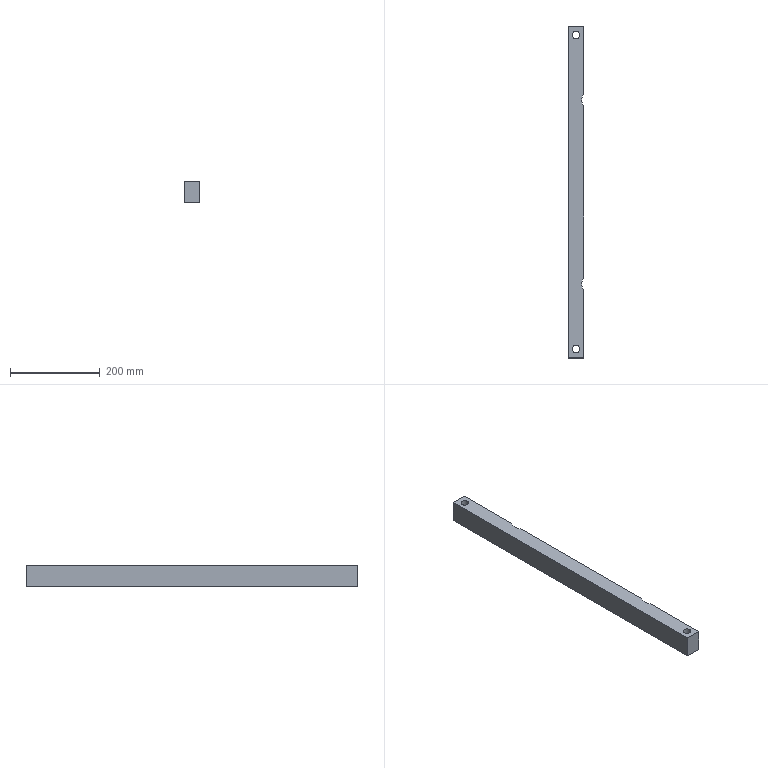Part | NX | features solid 2 | 1 solid | 12 faces | box 35 x 740 x 49 mm | volume 1237665 mm3 | plane 8 | cylinder 4 | commonest cylinder face diameters 17 x2 57 x2
STEP:
#1=CARTESIAN_POINT('',(510.5,-370.,153.));
#2=VERTEX_POINT('',#1);
#3=CARTESIAN_POINT('',(510.5,-370.,202.));
#4=VERTEX_POINT('',#3);
#5=CARTESIAN_POINT('',(510.5,-370.,148.));
#6=DIRECTION('',(0.,0.,1.));
#7=VECTOR('',#6,1000.);
#8=LINE('',#5,#7);
#9=EDGE_CURVE('',#2,#4,#8,.T.);
#10=ORIENTED_EDGE('',*,*,#9,.F.);
#11=CARTESIAN_POINT('',(510.5,-220.37,153.));
#12=VERTEX_POINT('',#11);
#13=CARTESIAN_POINT('',(510.5,0.,153.));
#14=DIRECTION('',(0.,1.,0.));
#15=VECTOR('',#14,1000.);
#16=LINE('',#13,#15);
#17=EDGE_CURVE('',#2,#12,#16,.T.);
#18=ORIENTED_EDGE('',*,*,#17,.T.);
#19=CARTESIAN_POINT('',(510.5,-220.37,202.));
#20=VERTEX_POINT('',#19);
#21=CARTESIAN_POINT('',(510.5,-220.37,308.));
#22=DIRECTION('',(0.,0.,-1.));
#23=VECTOR('',#22,1000.);
#24=LINE('',#21,#23);
#25=EDGE_CURVE('',#12,#20,#24,.F.);
#26=ORIENTED_EDGE('',*,*,#25,.T.);
#27=CARTESIAN_POINT('',(510.5,0.,202.));
#28=DIRECTION('',(0.,-1.,0.));
#29=VECTOR('',#28,1000.);
#30=LINE('',#27,#29);
#31=EDGE_CURVE('',#20,#4,#30,.T.);
#32=ORIENTED_EDGE('',*,*,#31,.T.);
#33=EDGE_LOOP('',(#10,#18,#26,#32));
#34=FACE_BOUND('',#33,.T.);
#35=CARTESIAN_POINT('',(510.5,0.,148.));
#36=DIRECTION('',(1.,0.,0.));
#37=DIRECTION('',(0.,0.,-1.));
#38=AXIS2_PLACEMENT_3D('',#35,#36,#37);
#39=PLANE('',#38);
#40=ADVANCED_FACE('',(#34),#39,.T.);
#41=CARTESIAN_POINT('',(510.5,-189.63,202.));
#42=VERTEX_POINT('',#41);
#43=CARTESIAN_POINT('',(510.5,-189.63,153.));
#44=VERTEX_POINT('',#43);
#45=CARTESIAN_POINT('',(510.5,-189.63,308.));
#46=DIRECTION('',(0.,0.,-1.));
#47=VECTOR('',#46,1000.);
#48=LINE('',#45,#47);
#49=EDGE_CURVE('',#42,#44,#48,.T.);
#50=ORIENTED_EDGE('',*,*,#49,.T.);
#51=CARTESIAN_POINT('',(510.5,189.63,153.));
#52=VERTEX_POINT('',#51);
#53=CARTESIAN_POINT('',(510.5,0.,153.));
#54=DIRECTION('',(0.,1.,0.));
#55=VECTOR('',#54,1000.);
#56=LINE('',#53,#55);
#57=EDGE_CURVE('',#44,#52,#56,.T.);
#58=ORIENTED_EDGE('',*,*,#57,.T.);
#59=CARTESIAN_POINT('',(510.5,189.63,202.));
#60=VERTEX_POINT('',#59);
#61=CARTESIAN_POINT('',(510.5,189.63,308.));
#62=DIRECTION('',(0.,0.,-1.));
#63=VECTOR('',#62,1000.);
#64=LINE('',#61,#63);
#65=EDGE_CURVE('',#52,#60,#64,.F.);
#66=ORIENTED_EDGE('',*,*,#65,.T.);
#67=CARTESIAN_POINT('',(510.5,0.,202.));
#68=DIRECTION('',(0.,-1.,0.));
#69=VECTOR('',#68,1000.);
#70=LINE('',#67,#69);
#71=EDGE_CURVE('',#60,#42,#70,.T.);
#72=ORIENTED_EDGE('',*,*,#71,.T.);
#73=EDGE_LOOP('',(#50,#58,#66,#72));
#74=FACE_BOUND('',#73,.T.);
#75=CARTESIAN_POINT('',(510.5,0.,148.));
#76=DIRECTION('',(1.,0.,0.));
#77=DIRECTION('',(0.,0.,-1.));
#78=AXIS2_PLACEMENT_3D('',#75,#76,#77);
#79=PLANE('',#78);
#80=ADVANCED_FACE('',(#74),#79,.T.);
#81=CARTESIAN_POINT('',(510.5,220.37,202.));
#82=VERTEX_POINT('',#81);
#83=CARTESIAN_POINT('',(510.5,220.37,153.));
#84=VERTEX_POINT('',#83);
#85=CARTESIAN_POINT('',(510.5,220.37,308.));
#86=DIRECTION('',(0.,0.,-1.));
#87=VECTOR('',#86,1000.);
#88=LINE('',#85,#87);
#89=EDGE_CURVE('',#82,#84,#88,.T.);
#90=ORIENTED_EDGE('',*,*,#89,.T.);
#91=CARTESIAN_POINT('',(510.5,370.,153.));
#92=VERTEX_POINT('',#91);
#93=CARTESIAN_POINT('',(510.5,0.,153.));
#94=DIRECTION('',(0.,1.,0.));
#95=VECTOR('',#94,1000.);
#96=LINE('',#93,#95);
#97=EDGE_CURVE('',#84,#92,#96,.T.);
#98=ORIENTED_EDGE('',*,*,#97,.T.);
#99=CARTESIAN_POINT('',(510.5,370.,202.));
#100=VERTEX_POINT('',#99);
#101=CARTESIAN_POINT('',(510.5,370.,148.));
#102=DIRECTION('',(0.,0.,1.));
#103=VECTOR('',#102,1000.);
#104=LINE('',#101,#103);
#105=EDGE_CURVE('',#92,#100,#104,.T.);
#106=ORIENTED_EDGE('',*,*,#105,.T.);
#107=CARTESIAN_POINT('',(510.5,0.,202.));
#108=DIRECTION('',(0.,-1.,0.));
#109=VECTOR('',#108,1000.);
#110=LINE('',#107,#109);
#111=EDGE_CURVE('',#100,#82,#110,.T.);
#112=ORIENTED_EDGE('',*,*,#111,.T.);
#113=EDGE_LOOP('',(#90,#98,#106,#112));
#114=FACE_BOUND('',#113,.T.);
#115=CARTESIAN_POINT('',(510.5,0.,148.));
#116=DIRECTION('',(1.,0.,0.));
#117=DIRECTION('',(0.,0.,-1.));
#118=AXIS2_PLACEMENT_3D('',#115,#116,#117);
#119=PLANE('',#118);
#120=ADVANCED_FACE('',(#114),#119,.T.);
#121=CARTESIAN_POINT('',(484.5,-350.,202.));
#122=VERTEX_POINT('',#121);
#123=CARTESIAN_POINT('',(493.,-350.,202.));
#124=DIRECTION('',(0.,0.,1.));
#125=DIRECTION('',(-1.,0.,0.));
#126=AXIS2_PLACEMENT_3D('',#123,#124,#125);
#127=CIRCLE('',#126,8.5);
#128=EDGE_CURVE('',#122,#122,#127,.F.);
#129=ORIENTED_EDGE('',*,*,#128,.F.);
#130=EDGE_LOOP('',(#129));
#131=FACE_BOUND('',#130,.T.);
#132=CARTESIAN_POINT('',(484.5,-350.,153.));
#133=VERTEX_POINT('',#132);
#134=CARTESIAN_POINT('',(493.,-350.,153.));
#135=DIRECTION('',(0.,0.,-1.));
#136=DIRECTION('',(-1.,0.,0.));
#137=AXIS2_PLACEMENT_3D('',#134,#135,#136);
#138=CIRCLE('',#137,8.5);
#139=EDGE_CURVE('',#133,#133,#138,.F.);
#140=ORIENTED_EDGE('',*,*,#139,.F.);
#141=EDGE_LOOP('',(#140));
#142=FACE_BOUND('',#141,.T.);
#143=CARTESIAN_POINT('',(493.,-350.,202.));
#144=DIRECTION('',(0.,0.,-1.));
#145=DIRECTION('',(-1.,0.,0.));
#146=AXIS2_PLACEMENT_3D('',#143,#144,#145);
#147=CYLINDRICAL_SURFACE('',#146,8.5);
#148=ADVANCED_FACE('',(#131,#142),#147,.F.);
#149=CARTESIAN_POINT('',(475.5,370.,153.));
#150=VERTEX_POINT('',#149);
#151=CARTESIAN_POINT('',(475.5,370.,202.));
#152=VERTEX_POINT('',#151);
#153=CARTESIAN_POINT('',(475.5,370.,148.));
#154=DIRECTION('',(0.,0.,1.));
#155=VECTOR('',#154,1000.);
#156=LINE('',#153,#155);
#157=EDGE_CURVE('',#150,#152,#156,.T.);
#158=ORIENTED_EDGE('',*,*,#157,.F.);
#159=CARTESIAN_POINT('',(475.5,-370.,153.));
#160=VERTEX_POINT('',#159);
#161=CARTESIAN_POINT('',(475.5,0.,153.));
#162=DIRECTION('',(0.,-1.,0.));
#163=VECTOR('',#162,1000.);
#164=LINE('',#161,#163);
#165=EDGE_CURVE('',#150,#160,#164,.T.);
#166=ORIENTED_EDGE('',*,*,#165,.T.);
#167=CARTESIAN_POINT('',(475.5,-370.,202.));
#168=VERTEX_POINT('',#167);
#169=CARTESIAN_POINT('',(475.5,-370.,148.));
#170=DIRECTION('',(0.,0.,1.));
#171=VECTOR('',#170,1000.);
#172=LINE('',#169,#171);
#173=EDGE_CURVE('',#160,#168,#172,.T.);
#174=ORIENTED_EDGE('',*,*,#173,.T.);
#175=CARTESIAN_POINT('',(475.5,0.,202.));
#176=DIRECTION('',(0.,1.,0.));
#177=VECTOR('',#176,1000.);
#178=LINE('',#175,#177);
#179=EDGE_CURVE('',#168,#152,#178,.T.);
#180=ORIENTED_EDGE('',*,*,#179,.T.);
#181=EDGE_LOOP('',(#158,#166,#174,#180));
#182=FACE_BOUND('',#181,.T.);
#183=CARTESIAN_POINT('',(475.5,0.,148.));
#184=DIRECTION('',(-1.,0.,0.));
#185=DIRECTION('',(0.,0.,1.));
#186=AXIS2_PLACEMENT_3D('',#183,#184,#185);
#187=PLANE('',#186);
#188=ADVANCED_FACE('',(#182),#187,.T.);
#189=ORIENTED_EDGE('',*,*,#105,.F.);
#190=CARTESIAN_POINT('',(493.,370.,153.));
#191=DIRECTION('',(-1.,0.,0.));
#192=VECTOR('',#191,1000.);
#193=LINE('',#190,#192);
#194=EDGE_CURVE('',#92,#150,#193,.T.);
#195=ORIENTED_EDGE('',*,*,#194,.T.);
#196=ORIENTED_EDGE('',*,*,#157,.T.);
#197=CARTESIAN_POINT('',(493.,370.,202.));
#198=DIRECTION('',(1.,0.,0.));
#199=VECTOR('',#198,1000.);
#200=LINE('',#197,#199);
#201=EDGE_CURVE('',#152,#100,#200,.T.);
#202=ORIENTED_EDGE('',*,*,#201,.T.);
#203=EDGE_LOOP('',(#189,#195,#196,#202));
#204=FACE_BOUND('',#203,.T.);
#205=CARTESIAN_POINT('',(493.,370.,148.));
#206=DIRECTION('',(0.,1.,0.));
#207=DIRECTION('',(0.,0.,1.));
#208=AXIS2_PLACEMENT_3D('',#205,#206,#207);
#209=PLANE('',#208);
#210=ADVANCED_FACE('',(#204),#209,.T.);
#211=ORIENTED_EDGE('',*,*,#173,.F.);
#212=CARTESIAN_POINT('',(493.,-370.,153.));
#213=DIRECTION('',(1.,0.,0.));
#214=VECTOR('',#213,1000.);
#215=LINE('',#212,#214);
#216=EDGE_CURVE('',#160,#2,#215,.T.);
#217=ORIENTED_EDGE('',*,*,#216,.T.);
#218=ORIENTED_EDGE('',*,*,#9,.T.);
#219=CARTESIAN_POINT('',(493.,-370.,202.));
#220=DIRECTION('',(-1.,0.,0.));
#221=VECTOR('',#220,1000.);
#222=LINE('',#219,#221);
#223=EDGE_CURVE('',#4,#168,#222,.T.);
#224=ORIENTED_EDGE('',*,*,#223,.T.);
#225=EDGE_LOOP('',(#211,#217,#218,#224));
#226=FACE_BOUND('',#225,.T.);
#227=CARTESIAN_POINT('',(493.,-370.,148.));
#228=DIRECTION('',(0.,-1.,0.));
#229=DIRECTION('',(0.,0.,-1.));
#230=AXIS2_PLACEMENT_3D('',#227,#228,#229);
#231=PLANE('',#230);
#232=ADVANCED_FACE('',(#226),#231,.T.);
#233=CARTESIAN_POINT('',(484.5,350.,202.));
#234=VERTEX_POINT('',#233);
#235=CARTESIAN_POINT('',(493.,350.,202.));
#236=DIRECTION('',(0.,0.,-1.));
#237=DIRECTION('',(-1.,0.,0.));
#238=AXIS2_PLACEMENT_3D('',#235,#236,#237);
#239=CIRCLE('',#238,8.5);
#240=EDGE_CURVE('',#234,#234,#239,.T.);
#241=ORIENTED_EDGE('',*,*,#240,.F.);
#242=EDGE_LOOP('',(#241));
#243=FACE_BOUND('',#242,.T.);
#244=CARTESIAN_POINT('',(484.5,350.,153.));
#245=VERTEX_POINT('',#244);
#246=CARTESIAN_POINT('',(493.,350.,153.));
#247=DIRECTION('',(0.,0.,-1.));
#248=DIRECTION('',(-1.,0.,0.));
#249=AXIS2_PLACEMENT_3D('',#246,#247,#248);
#250=CIRCLE('',#249,8.5);
#251=EDGE_CURVE('',#245,#245,#250,.F.);
#252=ORIENTED_EDGE('',*,*,#251,.F.);
#253=EDGE_LOOP('',(#252));
#254=FACE_BOUND('',#253,.T.);
#255=CARTESIAN_POINT('',(493.,350.,202.));
#256=DIRECTION('',(0.,0.,-1.));
#257=DIRECTION('',(-1.,0.,0.));
#258=AXIS2_PLACEMENT_3D('',#255,#256,#257);
#259=CYLINDRICAL_SURFACE('',#258,8.5);
#260=ADVANCED_FACE('',(#243,#254),#259,.F.);
#261=ORIENTED_EDGE('',*,*,#65,.F.);
#262=CARTESIAN_POINT('',(534.5,205.,153.));
#263=DIRECTION('',(0.,0.,-1.));
#264=DIRECTION('',(-1.,0.,0.));
#265=AXIS2_PLACEMENT_3D('',#262,#263,#264);
#266=CIRCLE('',#265,28.5);
#267=EDGE_CURVE('',#52,#84,#266,.T.);
#268=ORIENTED_EDGE('',*,*,#267,.T.);
#269=ORIENTED_EDGE('',*,*,#89,.F.);
#270=CARTESIAN_POINT('',(534.5,205.,202.));
#271=DIRECTION('',(0.,0.,1.));
#272=DIRECTION('',(1.,0.,0.));
#273=AXIS2_PLACEMENT_3D('',#270,#271,#272);
#274=CIRCLE('',#273,28.5);
#275=EDGE_CURVE('',#60,#82,#274,.F.);
#276=ORIENTED_EDGE('',*,*,#275,.F.);
#277=EDGE_LOOP('',(#261,#268,#269,#276));
#278=FACE_BOUND('',#277,.T.);
#279=CARTESIAN_POINT('',(534.5,205.,308.));
#280=DIRECTION('',(0.,0.,-1.));
#281=DIRECTION('',(-1.,0.,0.));
#282=AXIS2_PLACEMENT_3D('',#279,#280,#281);
#283=CYLINDRICAL_SURFACE('',#282,28.5);
#284=ADVANCED_FACE('',(#278),#283,.F.);
#285=ORIENTED_EDGE('',*,*,#25,.F.);
#286=CARTESIAN_POINT('',(534.5,-205.,153.));
#287=DIRECTION('',(0.,0.,-1.));
#288=DIRECTION('',(-1.,0.,0.));
#289=AXIS2_PLACEMENT_3D('',#286,#287,#288);
#290=CIRCLE('',#289,28.5);
#291=EDGE_CURVE('',#12,#44,#290,.T.);
#292=ORIENTED_EDGE('',*,*,#291,.T.);
#293=ORIENTED_EDGE('',*,*,#49,.F.);
#294=CARTESIAN_POINT('',(534.5,-205.,202.));
#295=DIRECTION('',(0.,0.,1.));
#296=DIRECTION('',(1.,0.,0.));
#297=AXIS2_PLACEMENT_3D('',#294,#295,#296);
#298=CIRCLE('',#297,28.5);
#299=EDGE_CURVE('',#20,#42,#298,.F.);
#300=ORIENTED_EDGE('',*,*,#299,.F.);
#301=EDGE_LOOP('',(#285,#292,#293,#300));
#302=FACE_BOUND('',#301,.T.);
#303=CARTESIAN_POINT('',(534.5,-205.,308.));
#304=DIRECTION('',(0.,0.,-1.));
#305=DIRECTION('',(-1.,0.,0.));
#306=AXIS2_PLACEMENT_3D('',#303,#304,#305);
#307=CYLINDRICAL_SURFACE('',#306,28.5);
#308=ADVANCED_FACE('',(#302),#307,.F.);
#309=ORIENTED_EDGE('',*,*,#128,.T.);
#310=EDGE_LOOP('',(#309));
#311=FACE_BOUND('',#310,.T.);
#312=ORIENTED_EDGE('',*,*,#240,.T.);
#313=EDGE_LOOP('',(#312));
#314=FACE_BOUND('',#313,.T.);
#315=ORIENTED_EDGE('',*,*,#31,.F.);
#316=ORIENTED_EDGE('',*,*,#299,.T.);
#317=ORIENTED_EDGE('',*,*,#71,.F.);
#318=ORIENTED_EDGE('',*,*,#275,.T.);
#319=ORIENTED_EDGE('',*,*,#111,.F.);
#320=ORIENTED_EDGE('',*,*,#201,.F.);
#321=ORIENTED_EDGE('',*,*,#179,.F.);
#322=ORIENTED_EDGE('',*,*,#223,.F.);
#323=EDGE_LOOP('',(#315,#316,#317,#318,#319,#320,#321,#322));
#324=FACE_BOUND('',#323,.T.);
#325=CARTESIAN_POINT('',(493.,0.,202.));
#326=DIRECTION('',(0.,0.,1.));
#327=DIRECTION('',(1.,0.,0.));
#328=AXIS2_PLACEMENT_3D('',#325,#326,#327);
#329=PLANE('',#328);
#330=ADVANCED_FACE('',(#311,#314,#324),#329,.T.);
#331=ORIENTED_EDGE('',*,*,#251,.T.);
#332=EDGE_LOOP('',(#331));
#333=FACE_BOUND('',#332,.T.);
#334=ORIENTED_EDGE('',*,*,#194,.F.);
#335=ORIENTED_EDGE('',*,*,#97,.F.);
#336=ORIENTED_EDGE('',*,*,#267,.F.);
#337=ORIENTED_EDGE('',*,*,#57,.F.);
#338=ORIENTED_EDGE('',*,*,#291,.F.);
#339=ORIENTED_EDGE('',*,*,#17,.F.);
#340=ORIENTED_EDGE('',*,*,#216,.F.);
#341=ORIENTED_EDGE('',*,*,#165,.F.);
#342=EDGE_LOOP('',(#334,#335,#336,#337,#338,#339,#340,#341));
#343=FACE_BOUND('',#342,.T.);
#344=ORIENTED_EDGE('',*,*,#139,.T.);
#345=EDGE_LOOP('',(#344));
#346=FACE_BOUND('',#345,.T.);
#347=CARTESIAN_POINT('',(835.5,0.,153.));
#348=DIRECTION('',(0.,0.,-1.));
#349=DIRECTION('',(-1.,0.,0.));
#350=AXIS2_PLACEMENT_3D('',#347,#348,#349);
#351=PLANE('',#350);
#352=ADVANCED_FACE('',(#333,#343,#346),#351,.T.);
#353=CLOSED_SHELL('',(#40,#80,#120,#148,#188,#210,#232,#260,#284,#308,#330,#352));
#354=MANIFOLD_SOLID_BREP('',#353);
#355=(LENGTH_UNIT()NAMED_UNIT(*)SI_UNIT(.MILLI.,.METRE.));
#356=UNCERTAINTY_MEASURE_WITH_UNIT(LENGTH_MEASURE(0.00001),#355,'','');
#357=(NAMED_UNIT(*)PLANE_ANGLE_UNIT()SI_UNIT($,.RADIAN.));
#358=(NAMED_UNIT(*)SI_UNIT($,.STERADIAN.)SOLID_ANGLE_UNIT());
#359=(GEOMETRIC_REPRESENTATION_CONTEXT(3)GLOBAL_UNCERTAINTY_ASSIGNED_CONTEXT((#356))GLOBAL_UNIT_ASSIGNED_CONTEXT((#355,#357,#358))REPRESENTATION_CONTEXT('',''));
#360=ADVANCED_BREP_SHAPE_REPRESENTATION('',(#354),#359);